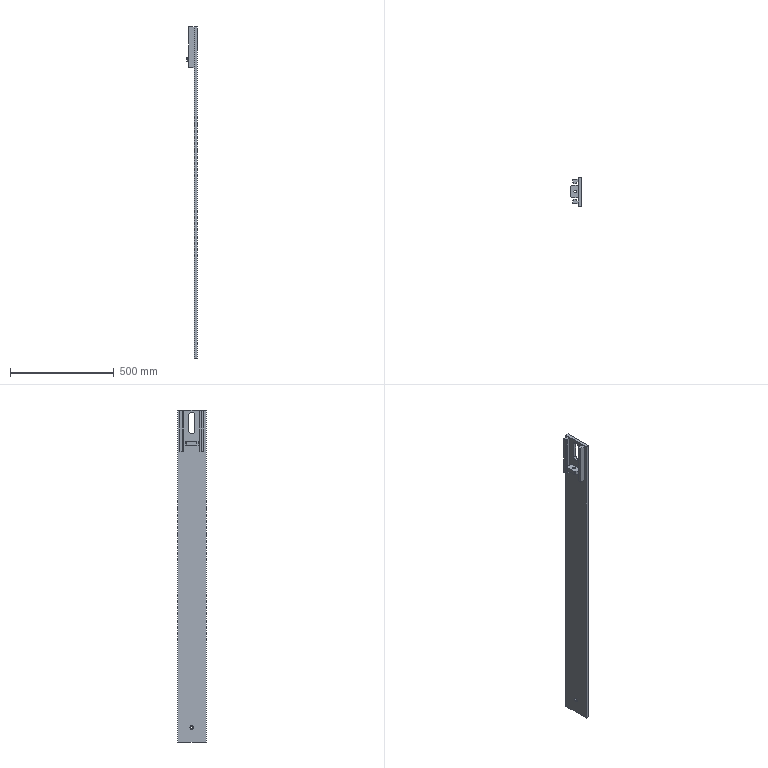Part | STEP file | PN_0012 | 3 solids | 44 faces | box 50 x 139 x 1600 mm | volume 3495566 mm3 | plane 36 | cylinder 8 | commonest cylinder face diameters 11 x2 12 x2 18 x2 30 x2